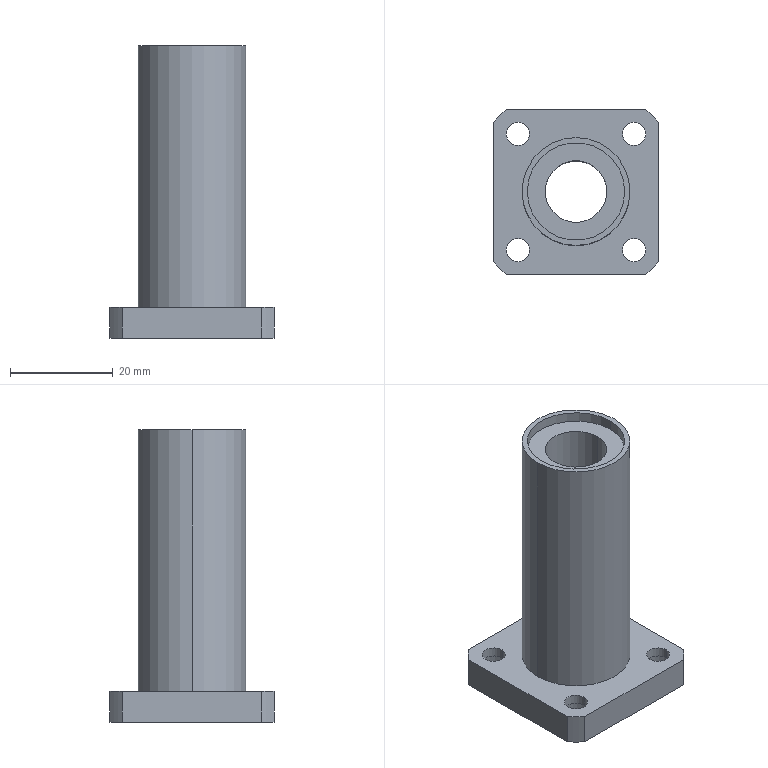Part | STEP file | 202-02-0006 | 1 solid | 41 faces | box 32 x 32 x 57 mm | volume 15769 mm3 | cylinder 28 | plane 13 | commonest cylinder face diameters 4.5 x8 7.5 x8 19 x4 42 x4 12 x2 21 x2